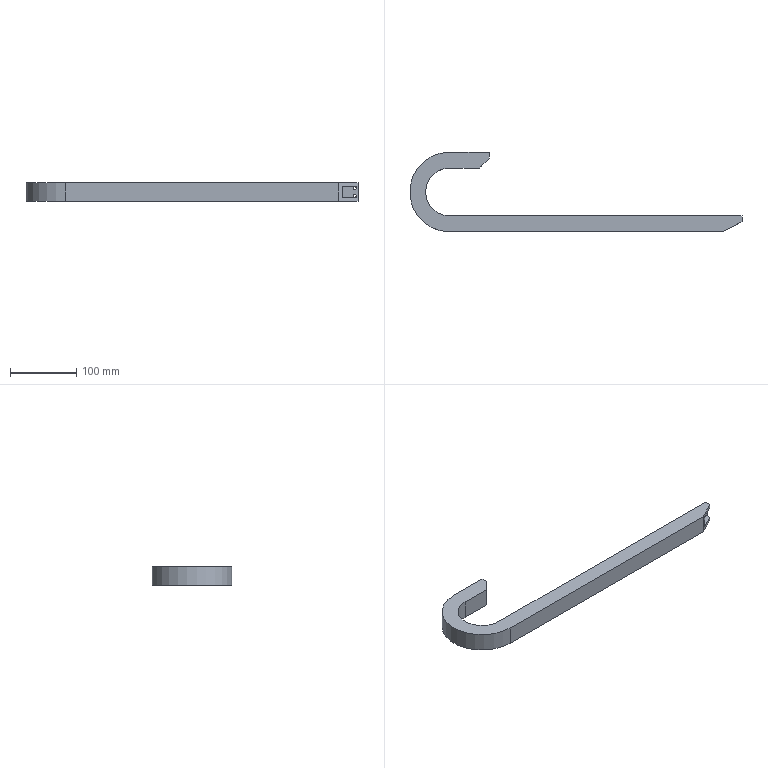Part | NX | 1 solid | 24 faces | box 500 x 120 x 28 mm | volume 220860 mm3 | plane 16 | cylinder 8 | commonest cylinder face diameters 4.5 x4 72 x1 78 x1 114 x1 120 x1
STEP:
#1=CARTESIAN_POINT('',(-392.,87.,-9.));
#2=VERTEX_POINT('',#1);
#3=CARTESIAN_POINT('',(-392.,87.,9.));
#4=VERTEX_POINT('',#3);
#5=CARTESIAN_POINT('',(-392.,87.,9.));
#6=DIRECTION('',(0.,0.,1.));
#7=VECTOR('',#6,1000.);
#8=LINE('',#5,#7);
#9=EDGE_CURVE('',#2,#4,#8,.T.);
#10=ORIENTED_EDGE('',*,*,#9,.F.);
#11=CARTESIAN_POINT('',(-440.,87.,-9.));
#12=VERTEX_POINT('',#11);
#13=CARTESIAN_POINT('',(-440.,87.,-9.));
#14=DIRECTION('',(1.,0.,0.));
#15=VECTOR('',#14,1000.);
#16=LINE('',#13,#15);
#17=EDGE_CURVE('',#12,#2,#16,.T.);
#18=ORIENTED_EDGE('',*,*,#17,.F.);
#19=CARTESIAN_POINT('',(-440.,87.,9.));
#20=VERTEX_POINT('',#19);
#21=CARTESIAN_POINT('',(-440.,87.,9.));
#22=DIRECTION('',(0.,0.,1.));
#23=VECTOR('',#22,1000.);
#24=LINE('',#21,#23);
#25=EDGE_CURVE('',#12,#20,#24,.T.);
#26=ORIENTED_EDGE('',*,*,#25,.T.);
#27=CARTESIAN_POINT('',(-440.,87.,9.));
#28=DIRECTION('',(1.,0.,0.));
#29=VECTOR('',#28,1000.);
#30=LINE('',#27,#29);
#31=EDGE_CURVE('',#20,#4,#30,.T.);
#32=ORIENTED_EDGE('',*,*,#31,.T.);
#33=EDGE_LOOP('',(#10,#18,#26,#32));
#34=FACE_BOUND('',#33,.T.);
#35=CARTESIAN_POINT('',(-440.,87.,9.));
#36=DIRECTION('',(0.,1.,0.));
#37=DIRECTION('',(-1.,0.,0.));
#38=AXIS2_PLACEMENT_3D('',#35,#36,#37);
#39=PLANE('',#38);
#40=ADVANCED_FACE('',(#34),#39,.T.);
#41=CARTESIAN_POINT('',(-385.,105.,3.75));
#42=VERTEX_POINT('',#41);
#43=CARTESIAN_POINT('',(-385.,105.,6.));
#44=DIRECTION('',(0.,-1.,0.));
#45=DIRECTION('',(0.,0.,-1.));
#46=AXIS2_PLACEMENT_3D('',#43,#44,#45);
#47=CIRCLE('',#46,2.25);
#48=EDGE_CURVE('',#42,#42,#47,.T.);
#49=ORIENTED_EDGE('',*,*,#48,.F.);
#50=EDGE_LOOP('',(#49));
#51=FACE_BOUND('',#50,.T.);
#52=CARTESIAN_POINT('',(-385.,105.,-8.25));
#53=VERTEX_POINT('',#52);
#54=CARTESIAN_POINT('',(-385.,105.,-6.));
#55=DIRECTION('',(0.,-1.,0.));
#56=DIRECTION('',(0.,0.,-1.));
#57=AXIS2_PLACEMENT_3D('',#54,#55,#56);
#58=CIRCLE('',#57,2.25);
#59=EDGE_CURVE('',#53,#53,#58,.T.);
#60=ORIENTED_EDGE('',*,*,#59,.F.);
#61=EDGE_LOOP('',(#60));
#62=FACE_BOUND('',#61,.T.);
#63=CARTESIAN_POINT('',(-440.,105.,9.));
#64=VERTEX_POINT('',#63);
#65=CARTESIAN_POINT('',(-440.,105.,-9.));
#66=VERTEX_POINT('',#65);
#67=CARTESIAN_POINT('',(-440.,105.,9.));
#68=DIRECTION('',(0.,0.,-1.));
#69=VECTOR('',#68,1000.);
#70=LINE('',#67,#69);
#71=EDGE_CURVE('',#64,#66,#70,.T.);
#72=ORIENTED_EDGE('',*,*,#71,.T.);
#73=CARTESIAN_POINT('',(-380.,105.,-9.));
#74=VERTEX_POINT('',#73);
#75=CARTESIAN_POINT('',(-440.,105.,-9.));
#76=DIRECTION('',(1.,0.,0.));
#77=VECTOR('',#76,1000.);
#78=LINE('',#75,#77);
#79=EDGE_CURVE('',#66,#74,#78,.T.);
#80=ORIENTED_EDGE('',*,*,#79,.T.);
#81=CARTESIAN_POINT('',(-380.,105.,9.));
#82=VERTEX_POINT('',#81);
#83=CARTESIAN_POINT('',(-380.,105.,9.));
#84=DIRECTION('',(0.,0.,-1.));
#85=VECTOR('',#84,1000.);
#86=LINE('',#83,#85);
#87=EDGE_CURVE('',#82,#74,#86,.T.);
#88=ORIENTED_EDGE('',*,*,#87,.F.);
#89=CARTESIAN_POINT('',(-440.,105.,9.));
#90=DIRECTION('',(1.,0.,0.));
#91=VECTOR('',#90,1000.);
#92=LINE('',#89,#91);
#93=EDGE_CURVE('',#64,#82,#92,.T.);
#94=ORIENTED_EDGE('',*,*,#93,.F.);
#95=EDGE_LOOP('',(#72,#80,#88,#94));
#96=FACE_BOUND('',#95,.T.);
#97=CARTESIAN_POINT('',(-440.,105.,9.));
#98=DIRECTION('',(0.,-1.,0.));
#99=DIRECTION('',(1.,0.,0.));
#100=AXIS2_PLACEMENT_3D('',#97,#98,#99);
#101=PLANE('',#100);
#102=ADVANCED_FACE('',(#51,#62,#96),#101,.T.);
#103=CARTESIAN_POINT('',(-385.,108.,3.75));
#104=VERTEX_POINT('',#103);
#105=CARTESIAN_POINT('',(-385.,108.,6.));
#106=DIRECTION('',(0.,-1.,0.));
#107=DIRECTION('',(0.,0.,-1.));
#108=AXIS2_PLACEMENT_3D('',#105,#106,#107);
#109=CIRCLE('',#108,2.25);
#110=EDGE_CURVE('',#104,#104,#109,.T.);
#111=ORIENTED_EDGE('',*,*,#110,.T.);
#112=EDGE_LOOP('',(#111));
#113=FACE_BOUND('',#112,.T.);
#114=CARTESIAN_POINT('',(-385.,108.,-8.25));
#115=VERTEX_POINT('',#114);
#116=CARTESIAN_POINT('',(-385.,108.,-6.));
#117=DIRECTION('',(0.,-1.,0.));
#118=DIRECTION('',(0.,0.,-1.));
#119=AXIS2_PLACEMENT_3D('',#116,#117,#118);
#120=CIRCLE('',#119,2.25);
#121=EDGE_CURVE('',#115,#115,#120,.T.);
#122=ORIENTED_EDGE('',*,*,#121,.T.);
#123=EDGE_LOOP('',(#122));
#124=FACE_BOUND('',#123,.T.);
#125=CARTESIAN_POINT('',(-440.,108.,14.));
#126=VERTEX_POINT('',#125);
#127=CARTESIAN_POINT('',(-440.,108.,-14.));
#128=VERTEX_POINT('',#127);
#129=CARTESIAN_POINT('',(-440.,108.,14.));
#130=DIRECTION('',(0.,0.,-1.));
#131=VECTOR('',#130,1000.);
#132=LINE('',#129,#131);
#133=EDGE_CURVE('',#126,#128,#132,.T.);
#134=ORIENTED_EDGE('',*,*,#133,.F.);
#135=CARTESIAN_POINT('',(-380.,108.,14.));
#136=VERTEX_POINT('',#135);
#137=CARTESIAN_POINT('',(-440.,108.,14.));
#138=DIRECTION('',(1.,0.,0.));
#139=VECTOR('',#138,1000.);
#140=LINE('',#137,#139);
#141=EDGE_CURVE('',#126,#136,#140,.T.);
#142=ORIENTED_EDGE('',*,*,#141,.T.);
#143=CARTESIAN_POINT('',(-380.,108.,-14.));
#144=VERTEX_POINT('',#143);
#145=CARTESIAN_POINT('',(-380.,108.,14.));
#146=DIRECTION('',(0.,0.,-1.));
#147=VECTOR('',#146,1000.);
#148=LINE('',#145,#147);
#149=EDGE_CURVE('',#136,#144,#148,.T.);
#150=ORIENTED_EDGE('',*,*,#149,.T.);
#151=CARTESIAN_POINT('',(-440.,108.,-14.));
#152=DIRECTION('',(1.,0.,0.));
#153=VECTOR('',#152,1000.);
#154=LINE('',#151,#153);
#155=EDGE_CURVE('',#128,#144,#154,.T.);
#156=ORIENTED_EDGE('',*,*,#155,.F.);
#157=EDGE_LOOP('',(#134,#142,#150,#156));
#158=FACE_BOUND('',#157,.T.);
#159=CARTESIAN_POINT('',(-440.,108.,14.));
#160=DIRECTION('',(0.,-1.,0.));
#161=DIRECTION('',(1.,0.,0.));
#162=AXIS2_PLACEMENT_3D('',#159,#160,#161);
#163=PLANE('',#162);
#164=ADVANCED_FACE('',(#113,#124,#158),#163,.F.);
#165=CARTESIAN_POINT('',(-440.,84.,-14.));
#166=VERTEX_POINT('',#165);
#167=CARTESIAN_POINT('',(-395.,84.,-14.));
#168=VERTEX_POINT('',#167);
#169=CARTESIAN_POINT('',(-440.,84.,-14.));
#170=DIRECTION('',(1.,0.,0.));
#171=VECTOR('',#170,1000.);
#172=LINE('',#169,#171);
#173=EDGE_CURVE('',#166,#168,#172,.T.);
#174=ORIENTED_EDGE('',*,*,#173,.T.);
#175=CARTESIAN_POINT('',(-395.,84.,14.));
#176=VERTEX_POINT('',#175);
#177=CARTESIAN_POINT('',(-395.,84.,14.));
#178=DIRECTION('',(0.,0.,-1.));
#179=VECTOR('',#178,1000.);
#180=LINE('',#177,#179);
#181=EDGE_CURVE('',#176,#168,#180,.T.);
#182=ORIENTED_EDGE('',*,*,#181,.F.);
#183=CARTESIAN_POINT('',(-440.,84.,14.));
#184=VERTEX_POINT('',#183);
#185=CARTESIAN_POINT('',(-440.,84.,14.));
#186=DIRECTION('',(1.,0.,0.));
#187=VECTOR('',#186,1000.);
#188=LINE('',#185,#187);
#189=EDGE_CURVE('',#184,#176,#188,.T.);
#190=ORIENTED_EDGE('',*,*,#189,.F.);
#191=CARTESIAN_POINT('',(-440.,84.,14.));
#192=DIRECTION('',(0.,0.,1.));
#193=VECTOR('',#192,1000.);
#194=LINE('',#191,#193);
#195=EDGE_CURVE('',#166,#184,#194,.T.);
#196=ORIENTED_EDGE('',*,*,#195,.F.);
#197=EDGE_LOOP('',(#174,#182,#190,#196));
#198=FACE_BOUND('',#197,.T.);
#199=CARTESIAN_POINT('',(-440.,84.,14.));
#200=DIRECTION('',(0.,1.,0.));
#201=DIRECTION('',(-1.,0.,0.));
#202=AXIS2_PLACEMENT_3D('',#199,#200,#201);
#203=PLANE('',#202);
#204=ADVANCED_FACE('',(#198),#203,.F.);
#205=CARTESIAN_POINT('',(-440.,9.,-9.));
#206=VERTEX_POINT('',#205);
#207=CARTESIAN_POINT('',(-440.,9.,9.));
#208=VERTEX_POINT('',#207);
#209=CARTESIAN_POINT('',(-440.,9.,9.));
#210=DIRECTION('',(0.,0.,1.));
#211=VECTOR('',#210,1000.);
#212=LINE('',#209,#211);
#213=EDGE_CURVE('',#206,#208,#212,.T.);
#214=ORIENTED_EDGE('',*,*,#213,.T.);
#215=CARTESIAN_POINT('',(-440.,48.,9.));
#216=DIRECTION('',(0.,0.,-1.));
#217=DIRECTION('',(-1.,0.,0.));
#218=AXIS2_PLACEMENT_3D('',#215,#216,#217);
#219=CIRCLE('',#218,39.);
#220=EDGE_CURVE('',#208,#20,#219,.T.);
#221=ORIENTED_EDGE('',*,*,#220,.T.);
#222=ORIENTED_EDGE('',*,*,#25,.F.);
#223=CARTESIAN_POINT('',(-440.,48.,-9.));
#224=DIRECTION('',(0.,0.,-1.));
#225=DIRECTION('',(-1.,0.,0.));
#226=AXIS2_PLACEMENT_3D('',#223,#224,#225);
#227=CIRCLE('',#226,39.);
#228=EDGE_CURVE('',#206,#12,#227,.T.);
#229=ORIENTED_EDGE('',*,*,#228,.F.);
#230=EDGE_LOOP('',(#214,#221,#222,#229));
#231=FACE_BOUND('',#230,.T.);
#232=CARTESIAN_POINT('',(-440.,48.,0.));
#233=DIRECTION('',(0.,0.,-1.));
#234=DIRECTION('',(-1.,0.,0.));
#235=AXIS2_PLACEMENT_3D('',#232,#233,#234);
#236=CYLINDRICAL_SURFACE('',#235,39.);
#237=ADVANCED_FACE('',(#231),#236,.T.);
#238=CARTESIAN_POINT('',(-440.,-9.,9.));
#239=VERTEX_POINT('',#238);
#240=CARTESIAN_POINT('',(-440.,-9.,-9.));
#241=VERTEX_POINT('',#240);
#242=CARTESIAN_POINT('',(-440.,-9.,9.));
#243=DIRECTION('',(0.,0.,-1.));
#244=VECTOR('',#243,1000.);
#245=LINE('',#242,#244);
#246=EDGE_CURVE('',#239,#241,#245,.T.);
#247=ORIENTED_EDGE('',*,*,#246,.T.);
#248=CARTESIAN_POINT('',(-440.,48.,-9.));
#249=DIRECTION('',(0.,0.,-1.));
#250=DIRECTION('',(-1.,0.,0.));
#251=AXIS2_PLACEMENT_3D('',#248,#249,#250);
#252=CIRCLE('',#251,57.);
#253=EDGE_CURVE('',#241,#66,#252,.T.);
#254=ORIENTED_EDGE('',*,*,#253,.T.);
#255=ORIENTED_EDGE('',*,*,#71,.F.);
#256=CARTESIAN_POINT('',(-440.,48.,9.));
#257=DIRECTION('',(0.,0.,-1.));
#258=DIRECTION('',(-1.,0.,0.));
#259=AXIS2_PLACEMENT_3D('',#256,#257,#258);
#260=CIRCLE('',#259,57.);
#261=EDGE_CURVE('',#239,#64,#260,.T.);
#262=ORIENTED_EDGE('',*,*,#261,.F.);
#263=EDGE_LOOP('',(#247,#254,#255,#262));
#264=FACE_BOUND('',#263,.T.);
#265=CARTESIAN_POINT('',(-440.,48.,0.));
#266=DIRECTION('',(0.,0.,-1.));
#267=DIRECTION('',(-1.,0.,0.));
#268=AXIS2_PLACEMENT_3D('',#265,#266,#267);
#269=CYLINDRICAL_SURFACE('',#268,57.);
#270=ADVANCED_FACE('',(#264),#269,.F.);
#271=CARTESIAN_POINT('',(-440.,-12.,14.));
#272=VERTEX_POINT('',#271);
#273=CARTESIAN_POINT('',(-440.,-12.,-14.));
#274=VERTEX_POINT('',#273);
#275=CARTESIAN_POINT('',(-440.,-12.,14.));
#276=DIRECTION('',(0.,0.,-1.));
#277=VECTOR('',#276,1000.);
#278=LINE('',#275,#277);
#279=EDGE_CURVE('',#272,#274,#278,.T.);
#280=ORIENTED_EDGE('',*,*,#279,.F.);
#281=CARTESIAN_POINT('',(-440.,48.,14.));
#282=DIRECTION('',(0.,0.,-1.));
#283=DIRECTION('',(-1.,0.,0.));
#284=AXIS2_PLACEMENT_3D('',#281,#282,#283);
#285=CIRCLE('',#284,60.);
#286=EDGE_CURVE('',#272,#126,#285,.T.);
#287=ORIENTED_EDGE('',*,*,#286,.T.);
#288=ORIENTED_EDGE('',*,*,#133,.T.);
#289=CARTESIAN_POINT('',(-440.,48.,-14.));
#290=DIRECTION('',(0.,0.,-1.));
#291=DIRECTION('',(-1.,0.,0.));
#292=AXIS2_PLACEMENT_3D('',#289,#290,#291);
#293=CIRCLE('',#292,60.);
#294=EDGE_CURVE('',#274,#128,#293,.T.);
#295=ORIENTED_EDGE('',*,*,#294,.F.);
#296=EDGE_LOOP('',(#280,#287,#288,#295));
#297=FACE_BOUND('',#296,.T.);
#298=CARTESIAN_POINT('',(-440.,48.,0.));
#299=DIRECTION('',(0.,0.,-1.));
#300=DIRECTION('',(-1.,0.,0.));
#301=AXIS2_PLACEMENT_3D('',#298,#299,#300);
#302=CYLINDRICAL_SURFACE('',#301,60.);
#303=ADVANCED_FACE('',(#297),#302,.T.);
#304=CARTESIAN_POINT('',(-440.,12.,-14.));
#305=VERTEX_POINT('',#304);
#306=CARTESIAN_POINT('',(-440.,12.,14.));
#307=VERTEX_POINT('',#306);
#308=CARTESIAN_POINT('',(-440.,12.,14.));
#309=DIRECTION('',(0.,0.,1.));
#310=VECTOR('',#309,1000.);
#311=LINE('',#308,#310);
#312=EDGE_CURVE('',#305,#307,#311,.T.);
#313=ORIENTED_EDGE('',*,*,#312,.F.);
#314=CARTESIAN_POINT('',(-440.,48.,-14.));
#315=DIRECTION('',(0.,0.,-1.));
#316=DIRECTION('',(-1.,0.,0.));
#317=AXIS2_PLACEMENT_3D('',#314,#315,#316);
#318=CIRCLE('',#317,36.);
#319=EDGE_CURVE('',#305,#166,#318,.T.);
#320=ORIENTED_EDGE('',*,*,#319,.T.);
#321=ORIENTED_EDGE('',*,*,#195,.T.);
#322=CARTESIAN_POINT('',(-440.,48.,14.));
#323=DIRECTION('',(0.,0.,-1.));
#324=DIRECTION('',(-1.,0.,0.));
#325=AXIS2_PLACEMENT_3D('',#322,#323,#324);
#326=CIRCLE('',#325,36.);
#327=EDGE_CURVE('',#307,#184,#326,.T.);
#328=ORIENTED_EDGE('',*,*,#327,.F.);
#329=EDGE_LOOP('',(#313,#320,#321,#328));
#330=FACE_BOUND('',#329,.T.);
#331=CARTESIAN_POINT('',(-440.,48.,0.));
#332=DIRECTION('',(0.,0.,-1.));
#333=DIRECTION('',(-1.,0.,0.));
#334=AXIS2_PLACEMENT_3D('',#331,#332,#333);
#335=CYLINDRICAL_SURFACE('',#334,36.);
#336=ADVANCED_FACE('',(#330),#335,.F.);
#337=CARTESIAN_POINT('',(-23.124,-9.,-9.));
#338=VERTEX_POINT('',#337);
#339=CARTESIAN_POINT('',(-440.,-9.,-9.));
#340=DIRECTION('',(1.,0.,0.));
#341=VECTOR('',#340,1000.);
#342=LINE('',#339,#341);
#343=EDGE_CURVE('',#241,#338,#342,.T.);
#344=ORIENTED_EDGE('',*,*,#343,.T.);
#345=CARTESIAN_POINT('',(0.,3.,-9.));
#346=VERTEX_POINT('',#345);
#347=CARTESIAN_POINT('',(-351.552,-179.437,-9.));
#348=DIRECTION('',(0.8876,0.4606,0.));
#349=VECTOR('',#348,1000.);
#350=LINE('',#347,#349);
#351=EDGE_CURVE('',#338,#346,#350,.T.);
#352=ORIENTED_EDGE('',*,*,#351,.T.);
#353=CARTESIAN_POINT('',(0.,9.,-9.));
#354=VERTEX_POINT('',#353);
#355=CARTESIAN_POINT('',(0.,-9.,-9.));
#356=DIRECTION('',(0.,1.,0.));
#357=VECTOR('',#356,1000.);
#358=LINE('',#355,#357);
#359=EDGE_CURVE('',#346,#354,#358,.T.);
#360=ORIENTED_EDGE('',*,*,#359,.T.);
#361=CARTESIAN_POINT('',(-440.,9.,-9.));
#362=DIRECTION('',(1.,0.,0.));
#363=VECTOR('',#362,1000.);
#364=LINE('',#361,#363);
#365=EDGE_CURVE('',#206,#354,#364,.T.);
#366=ORIENTED_EDGE('',*,*,#365,.F.);
#367=ORIENTED_EDGE('',*,*,#228,.T.);
#368=ORIENTED_EDGE('',*,*,#17,.T.);
#369=CARTESIAN_POINT('',(-380.,99.,-9.));
#370=VERTEX_POINT('',#369);
#371=CARTESIAN_POINT('',(-464.,15.,-9.));
#372=DIRECTION('',(0.7071,0.7071,0.));
#373=VECTOR('',#372,1000.);
#374=LINE('',#371,#373);
#375=EDGE_CURVE('',#2,#370,#374,.T.);
#376=ORIENTED_EDGE('',*,*,#375,.T.);
#377=CARTESIAN_POINT('',(-380.,105.,-9.));
#378=DIRECTION('',(0.,-1.,0.));
#379=VECTOR('',#378,1000.);
#380=LINE('',#377,#379);
#381=EDGE_CURVE('',#74,#370,#380,.T.);
#382=ORIENTED_EDGE('',*,*,#381,.F.);
#383=ORIENTED_EDGE('',*,*,#79,.F.);
#384=ORIENTED_EDGE('',*,*,#253,.F.);
#385=EDGE_LOOP('',(#344,#352,#360,#366,#367,#368,#376,#382,#383,#384));
#386=FACE_BOUND('',#385,.T.);
#387=CARTESIAN_POINT('',(-440.,-9.,-9.));
#388=DIRECTION('',(0.,0.,-1.));
#389=DIRECTION('',(-1.,0.,0.));
#390=AXIS2_PLACEMENT_3D('',#387,#388,#389);
#391=PLANE('',#390);
#392=ADVANCED_FACE('',(#386),#391,.F.);
#393=CARTESIAN_POINT('',(-7.25,9.,6.));
#394=VERTEX_POINT('',#393);
#395=CARTESIAN_POINT('',(-5.,9.,6.));
#396=DIRECTION('',(0.,1.,0.));
#397=DIRECTION('',(-1.,0.,0.));
#398=AXIS2_PLACEMENT_3D('',#395,#396,#397);
#399=CIRCLE('',#398,2.25);
#400=EDGE_CURVE('',#394,#394,#399,.T.);
#401=ORIENTED_EDGE('',*,*,#400,.T.);
#402=EDGE_LOOP('',(#401));
#403=FACE_BOUND('',#402,.T.);
#404=CARTESIAN_POINT('',(-7.25,9.,-6.));
#405=VERTEX_POINT('',#404);
#406=CARTESIAN_POINT('',(-5.,9.,-6.));
#407=DIRECTION('',(0.,1.,0.));
#408=DIRECTION('',(-1.,0.,0.));
#409=AXIS2_PLACEMENT_3D('',#406,#407,#408);
#410=CIRCLE('',#409,2.25);
#411=EDGE_CURVE('',#405,#405,#410,.T.);
#412=ORIENTED_EDGE('',*,*,#411,.T.);
#413=EDGE_LOOP('',(#412));
#414=FACE_BOUND('',#413,.T.);
#415=CARTESIAN_POINT('',(0.,9.,9.));
#416=VERTEX_POINT('',#415);
#417=CARTESIAN_POINT('',(0.,9.,9.));
#418=DIRECTION('',(0.,0.,1.));
#419=VECTOR('',#418,1000.);
#420=LINE('',#417,#419);
#421=EDGE_CURVE('',#354,#416,#420,.T.);
#422=ORIENTED_EDGE('',*,*,#421,.T.);
#423=CARTESIAN_POINT('',(-440.,9.,9.));
#424=DIRECTION('',(1.,0.,0.));
#425=VECTOR('',#424,1000.);
#426=LINE('',#423,#425);
#427=EDGE_CURVE('',#208,#416,#426,.T.);
#428=ORIENTED_EDGE('',*,*,#427,.F.);
#429=ORIENTED_EDGE('',*,*,#213,.F.);
#430=ORIENTED_EDGE('',*,*,#365,.T.);
#431=EDGE_LOOP('',(#422,#428,#429,#430));
#432=FACE_BOUND('',#431,.T.);
#433=CARTESIAN_POINT('',(-440.,9.,9.));
#434=DIRECTION('',(0.,1.,0.));
#435=DIRECTION('',(-1.,0.,0.));
#436=AXIS2_PLACEMENT_3D('',#433,#434,#435);
#437=PLANE('',#436);
#438=ADVANCED_FACE('',(#403,#414,#432),#437,.F.);
#439=CARTESIAN_POINT('',(0.,3.,9.));
#440=VERTEX_POINT('',#439);
#441=CARTESIAN_POINT('',(0.,-9.,9.));
#442=DIRECTION('',(0.,-1.,0.));
#443=VECTOR('',#442,1000.);
#444=LINE('',#441,#443);
#445=EDGE_CURVE('',#416,#440,#444,.T.);
#446=ORIENTED_EDGE('',*,*,#445,.T.);
#447=CARTESIAN_POINT('',(-23.124,-9.,9.));
#448=VERTEX_POINT('',#447);
#449=CARTESIAN_POINT('',(-351.552,-179.437,9.));
#450=DIRECTION('',(-0.8876,-0.4606,0.));
#451=VECTOR('',#450,1000.);
#452=LINE('',#449,#451);
#453=EDGE_CURVE('',#440,#448,#452,.T.);
#454=ORIENTED_EDGE('',*,*,#453,.T.);
#455=CARTESIAN_POINT('',(-440.,-9.,9.));
#456=DIRECTION('',(1.,0.,0.));
#457=VECTOR('',#456,1000.);
#458=LINE('',#455,#457);
#459=EDGE_CURVE('',#239,#448,#458,.T.);
#460=ORIENTED_EDGE('',*,*,#459,.F.);
#461=ORIENTED_EDGE('',*,*,#261,.T.);
#462=ORIENTED_EDGE('',*,*,#93,.T.);
#463=CARTESIAN_POINT('',(-380.,99.,9.));
#464=VERTEX_POINT('',#463);
#465=CARTESIAN_POINT('',(-380.,105.,9.));
#466=DIRECTION('',(0.,1.,0.));
#467=VECTOR('',#466,1000.);
#468=LINE('',#465,#467);
#469=EDGE_CURVE('',#464,#82,#468,.T.);
#470=ORIENTED_EDGE('',*,*,#469,.F.);
#471=CARTESIAN_POINT('',(-464.,15.,9.));
#472=DIRECTION('',(-0.7071,-0.7071,0.));
#473=VECTOR('',#472,1000.);
#474=LINE('',#471,#473);
#475=EDGE_CURVE('',#464,#4,#474,.T.);
#476=ORIENTED_EDGE('',*,*,#475,.T.);
#477=ORIENTED_EDGE('',*,*,#31,.F.);
#478=ORIENTED_EDGE('',*,*,#220,.F.);
#479=ORIENTED_EDGE('',*,*,#427,.T.);
#480=EDGE_LOOP('',(#446,#454,#460,#461,#462,#470,#476,#477,#478,#479));
#481=FACE_BOUND('',#480,.T.);
#482=CARTESIAN_POINT('',(-440.,-9.,9.));
#483=DIRECTION('',(0.,0.,1.));
#484=DIRECTION('',(1.,0.,0.));
#485=AXIS2_PLACEMENT_3D('',#482,#483,#484);
#486=PLANE('',#485);
#487=ADVANCED_FACE('',(#481),#486,.F.);
#488=CARTESIAN_POINT('',(0.,3.,-14.));
#489=VERTEX_POINT('',#488);
#490=CARTESIAN_POINT('',(-28.905,-12.,-14.));
#491=VERTEX_POINT('',#490);
#492=CARTESIAN_POINT('',(0.,3.,-14.));
#493=DIRECTION('',(-0.8876,-0.4606,0.));
#494=VECTOR('',#493,1000.);
#495=LINE('',#492,#494);
#496=EDGE_CURVE('',#489,#491,#495,.T.);
#497=ORIENTED_EDGE('',*,*,#496,.T.);
#498=CARTESIAN_POINT('',(-440.,-12.,-14.));
#499=DIRECTION('',(1.,0.,0.));
#500=VECTOR('',#499,1000.);
#501=LINE('',#498,#500);
#502=EDGE_CURVE('',#274,#491,#501,.T.);
#503=ORIENTED_EDGE('',*,*,#502,.F.);
#504=ORIENTED_EDGE('',*,*,#294,.T.);
#505=ORIENTED_EDGE('',*,*,#155,.T.);
#506=CARTESIAN_POINT('',(-380.,99.,-14.));
#507=VERTEX_POINT('',#506);
#508=CARTESIAN_POINT('',(-380.,108.,-14.));
#509=DIRECTION('',(0.,-1.,0.));
#510=VECTOR('',#509,1000.);
#511=LINE('',#508,#510);
#512=EDGE_CURVE('',#144,#507,#511,.T.);
#513=ORIENTED_EDGE('',*,*,#512,.T.);
#514=CARTESIAN_POINT('',(-380.,99.,-14.));
#515=DIRECTION('',(0.7071,0.7071,0.));
#516=VECTOR('',#515,1000.);
#517=LINE('',#514,#516);
#518=EDGE_CURVE('',#168,#507,#517,.T.);
#519=ORIENTED_EDGE('',*,*,#518,.F.);
#520=ORIENTED_EDGE('',*,*,#173,.F.);
#521=ORIENTED_EDGE('',*,*,#319,.F.);
#522=CARTESIAN_POINT('',(0.,12.,-14.));
#523=VERTEX_POINT('',#522);
#524=CARTESIAN_POINT('',(-440.,12.,-14.));
#525=DIRECTION('',(1.,0.,0.));
#526=VECTOR('',#525,1000.);
#527=LINE('',#524,#526);
#528=EDGE_CURVE('',#305,#523,#527,.T.);
#529=ORIENTED_EDGE('',*,*,#528,.T.);
#530=CARTESIAN_POINT('',(0.,-12.,-14.));
#531=DIRECTION('',(0.,1.,0.));
#532=VECTOR('',#531,1000.);
#533=LINE('',#530,#532);
#534=EDGE_CURVE('',#489,#523,#533,.T.);
#535=ORIENTED_EDGE('',*,*,#534,.F.);
#536=EDGE_LOOP('',(#497,#503,#504,#505,#513,#519,#520,#521,#529,#535));
#537=FACE_BOUND('',#536,.T.);
#538=CARTESIAN_POINT('',(-440.,-12.,-14.));
#539=DIRECTION('',(0.,0.,-1.));
#540=DIRECTION('',(-1.,0.,0.));
#541=AXIS2_PLACEMENT_3D('',#538,#539,#540);
#542=PLANE('',#541);
#543=ADVANCED_FACE('',(#537),#542,.T.);
#544=CARTESIAN_POINT('',(-28.905,-12.,14.));
#545=VERTEX_POINT('',#544);
#546=CARTESIAN_POINT('',(-28.905,-12.,-14.));
#547=DIRECTION('',(0.,0.,1.));
#548=VECTOR('',#547,1000.);
#549=LINE('',#546,#548);
#550=EDGE_CURVE('',#491,#545,#549,.T.);
#551=ORIENTED_EDGE('',*,*,#550,.T.);
#552=CARTESIAN_POINT('',(-440.,-12.,14.));
#553=DIRECTION('',(1.,0.,0.));
#554=VECTOR('',#553,1000.);
#555=LINE('',#552,#554);
#556=EDGE_CURVE('',#272,#545,#555,.T.);
#557=ORIENTED_EDGE('',*,*,#556,.F.);
#558=ORIENTED_EDGE('',*,*,#279,.T.);
#559=ORIENTED_EDGE('',*,*,#502,.T.);
#560=EDGE_LOOP('',(#551,#557,#558,#559));
#561=FACE_BOUND('',#560,.T.);
#562=CARTESIAN_POINT('',(-440.,-12.,14.));
#563=DIRECTION('',(0.,-1.,0.));
#564=DIRECTION('',(1.,0.,0.));
#565=AXIS2_PLACEMENT_3D('',#562,#563,#564);
#566=PLANE('',#565);
#567=ADVANCED_FACE('',(#561),#566,.T.);
#568=CARTESIAN_POINT('',(0.,3.,14.));
#569=VERTEX_POINT('',#568);
#570=CARTESIAN_POINT('',(0.,3.,14.));
#571=DIRECTION('',(-0.8876,-0.4606,0.));
#572=VECTOR('',#571,1000.);
#573=LINE('',#570,#572);
#574=EDGE_CURVE('',#569,#545,#573,.T.);
#575=ORIENTED_EDGE('',*,*,#574,.F.);
#576=CARTESIAN_POINT('',(0.,12.,14.));
#577=VERTEX_POINT('',#576);
#578=CARTESIAN_POINT('',(0.,-12.,14.));
#579=DIRECTION('',(0.,-1.,0.));
#580=VECTOR('',#579,1000.);
#581=LINE('',#578,#580);
#582=EDGE_CURVE('',#577,#569,#581,.T.);
#583=ORIENTED_EDGE('',*,*,#582,.F.);
#584=CARTESIAN_POINT('',(-440.,12.,14.));
#585=DIRECTION('',(1.,0.,0.));
#586=VECTOR('',#585,1000.);
#587=LINE('',#584,#586);
#588=EDGE_CURVE('',#307,#577,#587,.T.);
#589=ORIENTED_EDGE('',*,*,#588,.F.);
#590=ORIENTED_EDGE('',*,*,#327,.T.);
#591=ORIENTED_EDGE('',*,*,#189,.T.);
#592=CARTESIAN_POINT('',(-380.,99.,14.));
#593=VERTEX_POINT('',#592);
#594=CARTESIAN_POINT('',(-380.,99.,14.));
#595=DIRECTION('',(0.7071,0.7071,0.));
#596=VECTOR('',#595,1000.);
#597=LINE('',#594,#596);
#598=EDGE_CURVE('',#176,#593,#597,.T.);
#599=ORIENTED_EDGE('',*,*,#598,.T.);
#600=CARTESIAN_POINT('',(-380.,108.,14.));
#601=DIRECTION('',(0.,1.,0.));
#602=VECTOR('',#601,1000.);
#603=LINE('',#600,#602);
#604=EDGE_CURVE('',#593,#136,#603,.T.);
#605=ORIENTED_EDGE('',*,*,#604,.T.);
#606=ORIENTED_EDGE('',*,*,#141,.F.);
#607=ORIENTED_EDGE('',*,*,#286,.F.);
#608=ORIENTED_EDGE('',*,*,#556,.T.);
#609=EDGE_LOOP('',(#575,#583,#589,#590,#591,#599,#605,#606,#607,#608));
#610=FACE_BOUND('',#609,.T.);
#611=CARTESIAN_POINT('',(-440.,-12.,14.));
#612=DIRECTION('',(0.,0.,1.));
#613=DIRECTION('',(1.,0.,0.));
#614=AXIS2_PLACEMENT_3D('',#611,#612,#613);
#615=PLANE('',#614);
#616=ADVANCED_FACE('',(#610),#615,.T.);
#617=CARTESIAN_POINT('',(-7.25,12.,6.));
#618=VERTEX_POINT('',#617);
#619=CARTESIAN_POINT('',(-5.,12.,6.));
#620=DIRECTION('',(0.,1.,0.));
#621=DIRECTION('',(-1.,0.,0.));
#622=AXIS2_PLACEMENT_3D('',#619,#620,#621);
#623=CIRCLE('',#622,2.25);
#624=EDGE_CURVE('',#618,#618,#623,.T.);
#625=ORIENTED_EDGE('',*,*,#624,.F.);
#626=EDGE_LOOP('',(#625));
#627=FACE_BOUND('',#626,.T.);
#628=CARTESIAN_POINT('',(-7.25,12.,-6.));
#629=VERTEX_POINT('',#628);
#630=CARTESIAN_POINT('',(-5.,12.,-6.));
#631=DIRECTION('',(0.,1.,0.));
#632=DIRECTION('',(-1.,0.,0.));
#633=AXIS2_PLACEMENT_3D('',#630,#631,#632);
#634=CIRCLE('',#633,2.25);
#635=EDGE_CURVE('',#629,#629,#634,.T.);
#636=ORIENTED_EDGE('',*,*,#635,.F.);
#637=EDGE_LOOP('',(#636));
#638=FACE_BOUND('',#637,.T.);
#639=CARTESIAN_POINT('',(0.,12.,14.));
#640=DIRECTION('',(0.,0.,1.));
#641=VECTOR('',#640,1000.);
#642=LINE('',#639,#641);
#643=EDGE_CURVE('',#523,#577,#642,.T.);
#644=ORIENTED_EDGE('',*,*,#643,.F.);
#645=ORIENTED_EDGE('',*,*,#528,.F.);
#646=ORIENTED_EDGE('',*,*,#312,.T.);
#647=ORIENTED_EDGE('',*,*,#588,.T.);
#648=EDGE_LOOP('',(#644,#645,#646,#647));
#649=FACE_BOUND('',#648,.T.);
#650=CARTESIAN_POINT('',(-440.,12.,14.));
#651=DIRECTION('',(0.,1.,0.));
#652=DIRECTION('',(-1.,0.,0.));
#653=AXIS2_PLACEMENT_3D('',#650,#651,#652);
#654=PLANE('',#653);
#655=ADVANCED_FACE('',(#627,#638,#649),#654,.T.);
#656=ORIENTED_EDGE('',*,*,#459,.T.);
#657=CARTESIAN_POINT('',(-23.124,-9.,9.));
#658=DIRECTION('',(0.,0.,-1.));
#659=VECTOR('',#658,1000.);
#660=LINE('',#657,#659);
#661=EDGE_CURVE('',#448,#338,#660,.T.);
#662=ORIENTED_EDGE('',*,*,#661,.T.);
#663=ORIENTED_EDGE('',*,*,#343,.F.);
#664=ORIENTED_EDGE('',*,*,#246,.F.);
#665=EDGE_LOOP('',(#656,#662,#663,#664));
#666=FACE_BOUND('',#665,.T.);
#667=CARTESIAN_POINT('',(-440.,-9.,9.));
#668=DIRECTION('',(0.,-1.,0.));
#669=DIRECTION('',(1.,0.,0.));
#670=AXIS2_PLACEMENT_3D('',#667,#668,#669);
#671=PLANE('',#670);
#672=ADVANCED_FACE('',(#666),#671,.F.);
#673=CARTESIAN_POINT('',(-380.,99.,0.));
#674=DIRECTION('',(0.,0.,1.));
#675=VECTOR('',#674,1000.);
#676=LINE('',#673,#675);
#677=EDGE_CURVE('',#370,#507,#676,.F.);
#678=ORIENTED_EDGE('',*,*,#677,.T.);
#679=ORIENTED_EDGE('',*,*,#512,.F.);
#680=ORIENTED_EDGE('',*,*,#149,.F.);
#681=ORIENTED_EDGE('',*,*,#604,.F.);
#682=CARTESIAN_POINT('',(-380.,99.,14.));
#683=DIRECTION('',(0.,0.,-1.));
#684=VECTOR('',#683,1000.);
#685=LINE('',#682,#684);
#686=EDGE_CURVE('',#593,#464,#685,.T.);
#687=ORIENTED_EDGE('',*,*,#686,.T.);
#688=ORIENTED_EDGE('',*,*,#469,.T.);
#689=ORIENTED_EDGE('',*,*,#87,.T.);
#690=ORIENTED_EDGE('',*,*,#381,.T.);
#691=EDGE_LOOP('',(#678,#679,#680,#681,#687,#688,#689,#690));
#692=FACE_BOUND('',#691,.T.);
#693=CARTESIAN_POINT('',(-380.,96.,0.));
#694=DIRECTION('',(1.,0.,0.));
#695=DIRECTION('',(0.,0.,1.));
#696=AXIS2_PLACEMENT_3D('',#693,#694,#695);
#697=PLANE('',#696);
#698=ADVANCED_FACE('',(#692),#697,.T.);
#699=ORIENTED_EDGE('',*,*,#582,.T.);
#700=CARTESIAN_POINT('',(0.,3.,0.));
#701=DIRECTION('',(0.,0.,-1.));
#702=VECTOR('',#701,1000.);
#703=LINE('',#700,#702);
#704=EDGE_CURVE('',#569,#440,#703,.T.);
#705=ORIENTED_EDGE('',*,*,#704,.T.);
#706=ORIENTED_EDGE('',*,*,#445,.F.);
#707=ORIENTED_EDGE('',*,*,#421,.F.);
#708=ORIENTED_EDGE('',*,*,#359,.F.);
#709=CARTESIAN_POINT('',(0.,3.,-14.));
#710=DIRECTION('',(0.,0.,1.));
#711=VECTOR('',#710,1000.);
#712=LINE('',#709,#711);
#713=EDGE_CURVE('',#346,#489,#712,.F.);
#714=ORIENTED_EDGE('',*,*,#713,.T.);
#715=ORIENTED_EDGE('',*,*,#534,.T.);
#716=ORIENTED_EDGE('',*,*,#643,.T.);
#717=EDGE_LOOP('',(#699,#705,#706,#707,#708,#714,#715,#716));
#718=FACE_BOUND('',#717,.T.);
#719=CARTESIAN_POINT('',(0.,0.,0.));
#720=DIRECTION('',(-1.,0.,0.));
#721=DIRECTION('',(0.,0.,1.));
#722=AXIS2_PLACEMENT_3D('',#719,#720,#721);
#723=PLANE('',#722);
#724=ADVANCED_FACE('',(#718),#723,.F.);
#725=ORIENTED_EDGE('',*,*,#9,.T.);
#726=ORIENTED_EDGE('',*,*,#475,.F.);
#727=ORIENTED_EDGE('',*,*,#686,.F.);
#728=ORIENTED_EDGE('',*,*,#598,.F.);
#729=ORIENTED_EDGE('',*,*,#181,.T.);
#730=ORIENTED_EDGE('',*,*,#518,.T.);
#731=ORIENTED_EDGE('',*,*,#677,.F.);
#732=ORIENTED_EDGE('',*,*,#375,.F.);
#733=EDGE_LOOP('',(#725,#726,#727,#728,#729,#730,#731,#732));
#734=FACE_BOUND('',#733,.T.);
#735=CARTESIAN_POINT('',(-380.,99.,14.));
#736=DIRECTION('',(-0.7071,0.7071,0.));
#737=DIRECTION('',(-0.7071,-0.7071,0.));
#738=AXIS2_PLACEMENT_3D('',#735,#736,#737);
#739=PLANE('',#738);
#740=ADVANCED_FACE('',(#734),#739,.F.);
#741=ORIENTED_EDGE('',*,*,#661,.F.);
#742=ORIENTED_EDGE('',*,*,#453,.F.);
#743=ORIENTED_EDGE('',*,*,#704,.F.);
#744=ORIENTED_EDGE('',*,*,#574,.T.);
#745=ORIENTED_EDGE('',*,*,#550,.F.);
#746=ORIENTED_EDGE('',*,*,#496,.F.);
#747=ORIENTED_EDGE('',*,*,#713,.F.);
#748=ORIENTED_EDGE('',*,*,#351,.F.);
#749=EDGE_LOOP('',(#741,#742,#743,#744,#745,#746,#747,#748));
#750=FACE_BOUND('',#749,.T.);
#751=CARTESIAN_POINT('',(0.,3.,-14.));
#752=DIRECTION('',(-0.4606,0.8876,0.));
#753=DIRECTION('',(-0.8876,-0.4606,0.));
#754=AXIS2_PLACEMENT_3D('',#751,#752,#753);
#755=PLANE('',#754);
#756=ADVANCED_FACE('',(#750),#755,.F.);
#757=ORIENTED_EDGE('',*,*,#635,.T.);
#758=EDGE_LOOP('',(#757));
#759=FACE_BOUND('',#758,.T.);
#760=ORIENTED_EDGE('',*,*,#411,.F.);
#761=EDGE_LOOP('',(#760));
#762=FACE_BOUND('',#761,.T.);
#763=CARTESIAN_POINT('',(-5.,-9.,-6.));
#764=DIRECTION('',(0.,-1.,0.));
#765=DIRECTION('',(0.,0.,-1.));
#766=AXIS2_PLACEMENT_3D('',#763,#764,#765);
#767=CYLINDRICAL_SURFACE('',#766,2.25);
#768=ADVANCED_FACE('',(#759,#762),#767,.F.);
#769=ORIENTED_EDGE('',*,*,#624,.T.);
#770=EDGE_LOOP('',(#769));
#771=FACE_BOUND('',#770,.T.);
#772=ORIENTED_EDGE('',*,*,#400,.F.);
#773=EDGE_LOOP('',(#772));
#774=FACE_BOUND('',#773,.T.);
#775=CARTESIAN_POINT('',(-5.,-9.,6.));
#776=DIRECTION('',(0.,-1.,0.));
#777=DIRECTION('',(0.,0.,-1.));
#778=AXIS2_PLACEMENT_3D('',#775,#776,#777);
#779=CYLINDRICAL_SURFACE('',#778,2.25);
#780=ADVANCED_FACE('',(#771,#774),#779,.F.);
#781=ORIENTED_EDGE('',*,*,#121,.F.);
#782=EDGE_LOOP('',(#781));
#783=FACE_BOUND('',#782,.T.);
#784=ORIENTED_EDGE('',*,*,#59,.T.);
#785=EDGE_LOOP('',(#784));
#786=FACE_BOUND('',#785,.T.);
#787=CARTESIAN_POINT('',(-385.,105.,-6.));
#788=DIRECTION('',(0.,-1.,0.));
#789=DIRECTION('',(0.,0.,-1.));
#790=AXIS2_PLACEMENT_3D('',#787,#788,#789);
#791=CYLINDRICAL_SURFACE('',#790,2.25);
#792=ADVANCED_FACE('',(#783,#786),#791,.F.);
#793=ORIENTED_EDGE('',*,*,#110,.F.);
#794=EDGE_LOOP('',(#793));
#795=FACE_BOUND('',#794,.T.);
#796=ORIENTED_EDGE('',*,*,#48,.T.);
#797=EDGE_LOOP('',(#796));
#798=FACE_BOUND('',#797,.T.);
#799=CARTESIAN_POINT('',(-385.,105.,6.));
#800=DIRECTION('',(0.,-1.,0.));
#801=DIRECTION('',(0.,0.,-1.));
#802=AXIS2_PLACEMENT_3D('',#799,#800,#801);
#803=CYLINDRICAL_SURFACE('',#802,2.25);
#804=ADVANCED_FACE('',(#795,#798),#803,.F.);
#805=CLOSED_SHELL('',(#40,#102,#164,#204,#237,#270,#303,#336,#392,#438,#487,#543,#567,#616,#655,#672,#698,#724,#740,#756,#768,#780,#792,#804));
#806=MANIFOLD_SOLID_BREP('',#805);
#807=(LENGTH_UNIT()NAMED_UNIT(*)SI_UNIT(.MILLI.,.METRE.));
#808=UNCERTAINTY_MEASURE_WITH_UNIT(LENGTH_MEASURE(0.00001),#807,'','');
#809=(NAMED_UNIT(*)PLANE_ANGLE_UNIT()SI_UNIT($,.RADIAN.));
#810=(NAMED_UNIT(*)SI_UNIT($,.STERADIAN.)SOLID_ANGLE_UNIT());
#811=(GEOMETRIC_REPRESENTATION_CONTEXT(3)GLOBAL_UNCERTAINTY_ASSIGNED_CONTEXT((#808))GLOBAL_UNIT_ASSIGNED_CONTEXT((#807,#809,#810))REPRESENTATION_CONTEXT('',''));
#812=ADVANCED_BREP_SHAPE_REPRESENTATION('',(#806),#811);